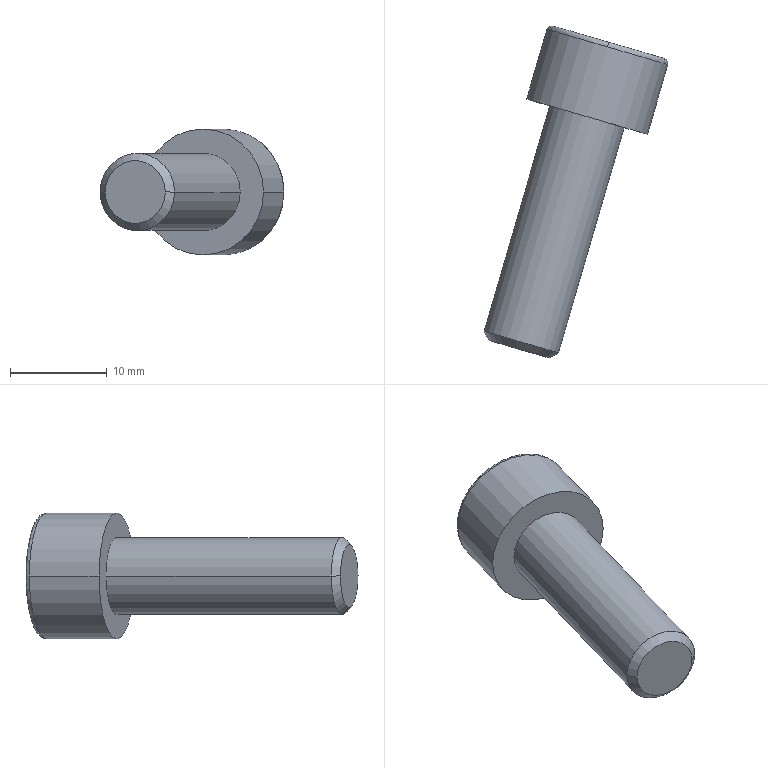Part | SolidWorks | features BaseBody 1 | 1 solid | 18 faces | box 18.984 x 34.285 x 13 mm | volume 2185 mm3 | plane 10 | cylinder 4 | cone 2 | spline 2 | commonest cylinder face diameters 8 x2 13 x2
STEP:
#1=CARTESIAN_POINT('',(22.625,457.214,-1.629));
#2=VERTEX_POINT('',#1);
#3=CARTESIAN_POINT('',(14.945,459.453,-1.629));
#4=VERTEX_POINT('',#3);
#5=CARTESIAN_POINT('',(18.785,458.333,-1.629));
#6=DIRECTION('',(-0.28,-0.96,0.));
#7=DIRECTION('',(0.96,-0.28,0.));
#8=AXIS2_PLACEMENT_3D('',#5,#6,#7);
#9=CIRCLE('',#8,4.);
#10=EDGE_CURVE('',#2,#4,#9,.T.);
#11=ORIENTED_EDGE('',*,*,#10,.T.);
#12=CARTESIAN_POINT('',(8.16,436.189,-1.629));
#13=VERTEX_POINT('',#12);
#14=CARTESIAN_POINT('',(11.553,447.821,-1.629));
#15=DIRECTION('',(-0.28,-0.96,0.));
#16=VECTOR('',#15,1000.);
#17=LINE('',#14,#16);
#18=EDGE_CURVE('',#4,#13,#17,.T.);
#19=ORIENTED_EDGE('',*,*,#18,.T.);
#20=CARTESIAN_POINT('',(15.841,433.95,-1.629));
#21=VERTEX_POINT('',#20);
#22=CARTESIAN_POINT('',(12.001,435.069,-1.629));
#23=DIRECTION('',(0.28,0.96,0.));
#24=DIRECTION('',(0.96,-0.28,0.));
#25=AXIS2_PLACEMENT_3D('',#22,#23,#24);
#26=CIRCLE('',#25,4.);
#27=EDGE_CURVE('',#13,#21,#26,.T.);
#28=ORIENTED_EDGE('',*,*,#27,.T.);
#29=CARTESIAN_POINT('',(19.233,445.582,-1.629));
#30=DIRECTION('',(-0.28,-0.96,0.));
#31=VECTOR('',#30,1000.);
#32=LINE('',#29,#31);
#33=EDGE_CURVE('',#2,#21,#32,.T.);
#34=ORIENTED_EDGE('',*,*,#33,.F.);
#35=EDGE_LOOP('',(#11,#19,#28,#34));
#36=FACE_OUTER_BOUND('',#35,.T.);
#37=CARTESIAN_POINT('',(15.393,446.701,-1.629));
#38=DIRECTION('',(-0.28,-0.96,0.));
#39=DIRECTION('',(0.96,-0.28,0.));
#40=AXIS2_PLACEMENT_3D('',#37,#38,#39);
#41=CYLINDRICAL_SURFACE('',#40,4.);
#42=ADVANCED_FACE('',(#36),#41,.T.);
#43=CARTESIAN_POINT('',(8.682,435.238,-1.629));
#44=VERTEX_POINT('',#43);
#45=CARTESIAN_POINT('',(14.89,433.428,-1.629));
#46=VERTEX_POINT('',#45);
#47=CARTESIAN_POINT('',(11.786,434.333,-1.629));
#48=DIRECTION('',(0.28,0.96,0.));
#49=DIRECTION('',(-0.96,0.28,0.));
#50=AXIS2_PLACEMENT_3D('',#47,#48,#49);
#51=CIRCLE('',#50,3.233);
#52=EDGE_CURVE('',#44,#46,#51,.T.);
#53=ORIENTED_EDGE('',*,*,#52,.T.);
#54=CARTESIAN_POINT('',(15.841,433.95,-1.629));
#55=DIRECTION('',(0.8768,0.4809,0.));
#56=VECTOR('',#55,1000.);
#57=LINE('',#54,#56);
#58=EDGE_CURVE('',#46,#21,#57,.T.);
#59=ORIENTED_EDGE('',*,*,#58,.T.);
#60=ORIENTED_EDGE('',*,*,#27,.F.);
#61=CARTESIAN_POINT('',(8.16,436.189,-1.629));
#62=DIRECTION('',(-0.4809,0.8768,0.));
#63=VECTOR('',#62,1000.);
#64=LINE('',#61,#63);
#65=EDGE_CURVE('',#44,#13,#64,.T.);
#66=ORIENTED_EDGE('',*,*,#65,.F.);
#67=EDGE_LOOP('',(#53,#59,#60,#66));
#68=FACE_OUTER_BOUND('',#67,.T.);
#69=CARTESIAN_POINT('',(12.001,435.069,-1.629));
#70=DIRECTION('',(0.28,0.96,0.));
#71=DIRECTION('',(-0.96,0.28,0.));
#72=AXIS2_PLACEMENT_3D('',#69,#70,#71);
#73=CONICAL_SURFACE('',#72,4.,0.7854);
#74=ADVANCED_FACE('',(#68),#73,.T.);
#75=CARTESIAN_POINT('',(20.884,465.534,4.871));
#76=VERTEX_POINT('',#75);
#77=CARTESIAN_POINT('',(14.644,467.353,-1.629));
#78=VERTEX_POINT('',#77);
#79=CARTESIAN_POINT('',(20.884,465.534,-1.629));
#80=DIRECTION('',(-0.28,-0.96,0.));
#81=DIRECTION('',(0.96,-0.28,0.));
#82=AXIS2_PLACEMENT_3D('',#79,#80,#81);
#83=CIRCLE('',#82,6.5);
#84=EDGE_CURVE('',#76,#78,#83,.T.);
#85=ORIENTED_EDGE('',*,*,#84,.T.);
#86=CARTESIAN_POINT('',(12.545,460.153,-1.629));
#87=VERTEX_POINT('',#86);
#88=CARTESIAN_POINT('',(13.594,463.753,-1.629));
#89=DIRECTION('',(-0.28,-0.96,0.));
#90=VECTOR('',#89,1000.);
#91=LINE('',#88,#90);
#92=EDGE_CURVE('',#78,#87,#91,.T.);
#93=ORIENTED_EDGE('',*,*,#92,.T.);
#94=CARTESIAN_POINT('',(25.025,456.514,-1.629));
#95=VERTEX_POINT('',#94);
#96=CARTESIAN_POINT('',(18.785,458.333,-1.629));
#97=DIRECTION('',(-0.28,-0.96,0.));
#98=DIRECTION('',(0.96,-0.28,0.));
#99=AXIS2_PLACEMENT_3D('',#96,#97,#98);
#100=CIRCLE('',#99,6.5);
#101=EDGE_CURVE('',#95,#87,#100,.T.);
#102=ORIENTED_EDGE('',*,*,#101,.F.);
#103=CARTESIAN_POINT('',(27.124,463.714,-1.629));
#104=VERTEX_POINT('',#103);
#105=CARTESIAN_POINT('',(26.075,460.114,-1.629));
#106=DIRECTION('',(-0.28,-0.96,0.));
#107=VECTOR('',#106,1000.);
#108=LINE('',#105,#107);
#109=EDGE_CURVE('',#104,#95,#108,.T.);
#110=ORIENTED_EDGE('',*,*,#109,.F.);
#111=CARTESIAN_POINT('',(20.884,465.534,-1.629));
#112=DIRECTION('',(-0.28,-0.96,0.));
#113=DIRECTION('',(0.96,-0.28,0.));
#114=AXIS2_PLACEMENT_3D('',#111,#112,#113);
#115=CIRCLE('',#114,6.5);
#116=EDGE_CURVE('',#104,#76,#115,.T.);
#117=ORIENTED_EDGE('',*,*,#116,.T.);
#118=EDGE_LOOP('',(#85,#93,#102,#110,#117));
#119=FACE_OUTER_BOUND('',#118,.T.);
#120=CARTESIAN_POINT('',(19.834,461.933,-1.629));
#121=DIRECTION('',(-0.28,-0.96,0.));
#122=DIRECTION('',(0.96,-0.28,0.));
#123=AXIS2_PLACEMENT_3D('',#120,#121,#122);
#124=CYLINDRICAL_SURFACE('',#123,6.5);
#125=ADVANCED_FACE('',(#119),#124,.T.);
#126=ORIENTED_EDGE('',*,*,#18,.F.);
#127=CARTESIAN_POINT('',(18.785,458.333,-1.629));
#128=DIRECTION('',(-0.28,-0.96,0.));
#129=DIRECTION('',(0.96,-0.28,0.));
#130=AXIS2_PLACEMENT_3D('',#127,#128,#129);
#131=CIRCLE('',#130,4.);
#132=EDGE_CURVE('',#4,#2,#131,.T.);
#133=ORIENTED_EDGE('',*,*,#132,.T.);
#134=ORIENTED_EDGE('',*,*,#33,.T.);
#135=CARTESIAN_POINT('',(12.001,435.069,-1.629));
#136=DIRECTION('',(0.28,0.96,0.));
#137=DIRECTION('',(0.96,-0.28,0.));
#138=AXIS2_PLACEMENT_3D('',#135,#136,#137);
#139=CIRCLE('',#138,4.);
#140=EDGE_CURVE('',#21,#13,#139,.T.);
#141=ORIENTED_EDGE('',*,*,#140,.T.);
#142=EDGE_LOOP('',(#126,#133,#134,#141));
#143=FACE_OUTER_BOUND('',#142,.T.);
#144=CARTESIAN_POINT('',(15.393,446.701,-1.629));
#145=DIRECTION('',(-0.28,-0.96,0.));
#146=DIRECTION('',(0.96,-0.28,0.));
#147=AXIS2_PLACEMENT_3D('',#144,#145,#146);
#148=CYLINDRICAL_SURFACE('',#147,4.);
#149=ADVANCED_FACE('',(#143),#148,.T.);
#150=ORIENTED_EDGE('',*,*,#58,.F.);
#151=CARTESIAN_POINT('',(11.786,434.333,-1.629));
#152=DIRECTION('',(0.28,0.96,0.));
#153=DIRECTION('',(-0.96,0.28,0.));
#154=AXIS2_PLACEMENT_3D('',#151,#152,#153);
#155=CIRCLE('',#154,3.233);
#156=EDGE_CURVE('',#46,#44,#155,.T.);
#157=ORIENTED_EDGE('',*,*,#156,.T.);
#158=ORIENTED_EDGE('',*,*,#65,.T.);
#159=ORIENTED_EDGE('',*,*,#140,.F.);
#160=EDGE_LOOP('',(#150,#157,#158,#159));
#161=FACE_OUTER_BOUND('',#160,.T.);
#162=CARTESIAN_POINT('',(12.001,435.069,-1.629));
#163=DIRECTION('',(0.28,0.96,0.));
#164=DIRECTION('',(-0.96,0.28,0.));
#165=AXIS2_PLACEMENT_3D('',#162,#163,#164);
#166=CONICAL_SURFACE('',#165,4.,0.7854);
#167=ADVANCED_FACE('',(#161),#166,.T.);
#168=ORIENTED_EDGE('',*,*,#101,.T.);
#169=CARTESIAN_POINT('',(18.785,458.333,-1.629));
#170=DIRECTION('',(-0.28,-0.96,0.));
#171=DIRECTION('',(0.96,-0.28,0.));
#172=AXIS2_PLACEMENT_3D('',#169,#170,#171);
#173=CIRCLE('',#172,6.5);
#174=EDGE_CURVE('',#87,#95,#173,.T.);
#175=ORIENTED_EDGE('',*,*,#174,.T.);
#176=EDGE_LOOP('',(#168,#175));
#177=FACE_OUTER_BOUND('',#176,.T.);
#178=ORIENTED_EDGE('',*,*,#10,.F.);
#179=ORIENTED_EDGE('',*,*,#132,.F.);
#180=EDGE_LOOP('',(#178,#179));
#181=FACE_BOUND('',#180,.T.);
#182=CARTESIAN_POINT('',(23.825,456.864,-1.629));
#183=DIRECTION('',(-0.28,-0.96,0.));
#184=DIRECTION('',(0.96,-0.28,0.));
#185=AXIS2_PLACEMENT_3D('',#182,#183,#184);
#186=PLANE('',#185);
#187=ADVANCED_FACE('',(#177,#181),#186,.T.);
#188=ORIENTED_EDGE('',*,*,#52,.F.);
#189=ORIENTED_EDGE('',*,*,#156,.F.);
#190=EDGE_LOOP('',(#188,#189));
#191=FACE_OUTER_BOUND('',#190,.T.);
#192=CARTESIAN_POINT('',(13.338,433.881,-1.629));
#193=DIRECTION('',(-0.28,-0.96,0.));
#194=DIRECTION('',(0.96,-0.28,0.));
#195=AXIS2_PLACEMENT_3D('',#192,#193,#194);
#196=PLANE('',#195);
#197=ADVANCED_FACE('',(#191),#196,.T.);
#198=ORIENTED_EDGE('',*,*,#92,.F.);
#199=CARTESIAN_POINT('',(20.884,465.534,-8.129));
#200=VERTEX_POINT('',#199);
#201=CARTESIAN_POINT('',(20.884,465.534,-1.629));
#202=DIRECTION('',(-0.28,-0.96,0.));
#203=DIRECTION('',(0.96,-0.28,0.));
#204=AXIS2_PLACEMENT_3D('',#201,#202,#203);
#205=CIRCLE('',#204,6.5);
#206=EDGE_CURVE('',#78,#200,#205,.T.);
#207=ORIENTED_EDGE('',*,*,#206,.T.);
#208=CARTESIAN_POINT('',(20.884,465.534,-1.629));
#209=DIRECTION('',(-0.28,-0.96,0.));
#210=DIRECTION('',(0.96,-0.28,0.));
#211=AXIS2_PLACEMENT_3D('',#208,#209,#210);
#212=CIRCLE('',#211,6.5);
#213=EDGE_CURVE('',#200,#104,#212,.T.);
#214=ORIENTED_EDGE('',*,*,#213,.T.);
#215=ORIENTED_EDGE('',*,*,#109,.T.);
#216=ORIENTED_EDGE('',*,*,#174,.F.);
#217=EDGE_LOOP('',(#198,#207,#214,#215,#216));
#218=FACE_OUTER_BOUND('',#217,.T.);
#219=CARTESIAN_POINT('',(19.834,461.933,-1.629));
#220=DIRECTION('',(-0.28,-0.96,0.));
#221=DIRECTION('',(0.96,-0.28,0.));
#222=AXIS2_PLACEMENT_3D('',#219,#220,#221);
#223=CYLINDRICAL_SURFACE('',#222,6.5);
#224=ADVANCED_FACE('',(#218),#223,.T.);
#225=ORIENTED_EDGE('',*,*,#84,.F.);
#226=CARTESIAN_POINT('',(21.024,466.014,4.371));
#227=VERTEX_POINT('',#226);
#228=CARTESIAN_POINT('',(20.884,465.534,4.871));
#229=CARTESIAN_POINT('',(20.966,465.815,4.871));
#230=CARTESIAN_POINT('',(21.024,466.014,4.664));
#231=CARTESIAN_POINT('',(21.024,466.014,4.371));
#232=(BOUNDED_CURVE()B_SPLINE_CURVE(3,(#228,#229,#230,#231),.UNSPECIFIED.,.F.,.F.)B_SPLINE_CURVE_WITH_KNOTS((4,4),(0.,1.455),.UNSPECIFIED.)CURVE()GEOMETRIC_REPRESENTATION_ITEM()RATIONAL_B_SPLINE_CURVE((1.,0.8047,0.8047,1.))REPRESENTATION_ITEM(''));
#233=EDGE_CURVE('',#76,#227,#232,.T.);
#234=ORIENTED_EDGE('',*,*,#233,.T.);
#235=CARTESIAN_POINT('',(21.024,466.014,-7.629));
#236=VERTEX_POINT('',#235);
#237=CARTESIAN_POINT('',(21.024,466.014,4.371));
#238=CARTESIAN_POINT('',(9.504,469.373,4.371));
#239=CARTESIAN_POINT('',(9.504,469.373,-7.629));
#240=CARTESIAN_POINT('',(21.024,466.014,-7.629));
#241=(BOUNDED_CURVE()B_SPLINE_CURVE(3,(#237,#238,#239,#240),.UNSPECIFIED.,.F.,.F.)B_SPLINE_CURVE_WITH_KNOTS((4,4),(0.,1.),.UNSPECIFIED.)CURVE()GEOMETRIC_REPRESENTATION_ITEM()RATIONAL_B_SPLINE_CURVE((1.,0.3333,0.3333,1.))REPRESENTATION_ITEM(''));
#242=EDGE_CURVE('',#227,#236,#241,.T.);
#243=ORIENTED_EDGE('',*,*,#242,.T.);
#244=CARTESIAN_POINT('',(21.024,466.014,-7.629));
#245=CARTESIAN_POINT('',(21.024,466.014,-7.922));
#246=CARTESIAN_POINT('',(20.966,465.815,-8.129));
#247=CARTESIAN_POINT('',(20.884,465.534,-8.129));
#248=(BOUNDED_CURVE()B_SPLINE_CURVE(3,(#244,#245,#246,#247),.UNSPECIFIED.,.F.,.F.)B_SPLINE_CURVE_WITH_KNOTS((4,4),(0.,1.455),.UNSPECIFIED.)CURVE()GEOMETRIC_REPRESENTATION_ITEM()RATIONAL_B_SPLINE_CURVE((1.,0.8047,0.8047,1.))REPRESENTATION_ITEM(''));
#249=EDGE_CURVE('',#236,#200,#248,.T.);
#250=ORIENTED_EDGE('',*,*,#249,.T.);
#251=ORIENTED_EDGE('',*,*,#206,.F.);
#252=EDGE_LOOP('',(#225,#234,#243,#250,#251));
#253=FACE_OUTER_BOUND('',#252,.T.);
#254=CARTESIAN_POINT('',(21.024,466.014,-7.629));
#255=CARTESIAN_POINT('',(9.504,469.373,-7.629));
#256=CARTESIAN_POINT('',(9.504,469.373,4.371));
#257=CARTESIAN_POINT('',(21.024,466.014,4.371));
#258=CARTESIAN_POINT('',(21.024,466.014,-7.922));
#259=CARTESIAN_POINT('',(8.942,469.537,-7.922));
#260=CARTESIAN_POINT('',(8.942,469.537,4.664));
#261=CARTESIAN_POINT('',(21.024,466.014,4.664));
#262=CARTESIAN_POINT('',(20.966,465.815,-8.129));
#263=CARTESIAN_POINT('',(8.486,469.454,-8.129));
#264=CARTESIAN_POINT('',(8.486,469.454,4.871));
#265=CARTESIAN_POINT('',(20.966,465.815,4.871));
#266=CARTESIAN_POINT('',(20.884,465.534,-8.129));
#267=CARTESIAN_POINT('',(8.404,469.173,-8.129));
#268=CARTESIAN_POINT('',(8.404,469.173,4.871));
#269=CARTESIAN_POINT('',(20.884,465.534,4.871));
#270=(BOUNDED_SURFACE()B_SPLINE_SURFACE(3,3,((#254,#255,#256,#257),(#258,#259,#260,#261),(#262,#263,#264,#265),(#266,#267,#268,#269)),.UNSPECIFIED.,.F.,.F.,.T.)B_SPLINE_SURFACE_WITH_KNOTS((4,4),(4,4),(0.,1.455),(0.,39.),.UNSPECIFIED.)GEOMETRIC_REPRESENTATION_ITEM()RATIONAL_B_SPLINE_SURFACE(((1.,0.3333,0.3333,1.),(0.8047,0.2682,0.2682,0.8047),(0.8047,0.2682,0.2682,0.8047),(1.,0.3333,0.3333,1.)))REPRESENTATION_ITEM('')SURFACE());
#271=ADVANCED_FACE('',(#253),#270,.T.);
#272=ORIENTED_EDGE('',*,*,#213,.F.);
#273=ORIENTED_EDGE('',*,*,#249,.F.);
#274=CARTESIAN_POINT('',(26.784,464.334,-1.629));
#275=VERTEX_POINT('',#274);
#276=CARTESIAN_POINT('',(21.024,466.014,-7.629));
#277=CARTESIAN_POINT('',(23.904,465.174,-7.629));
#278=CARTESIAN_POINT('',(26.784,464.334,-5.629));
#279=CARTESIAN_POINT('',(26.784,464.334,-1.629));
#280=(BOUNDED_CURVE()B_SPLINE_CURVE(3,(#276,#277,#278,#279),.UNSPECIFIED.,.F.,.F.)B_SPLINE_CURVE_WITH_KNOTS((4,4),(0.,1.),.UNSPECIFIED.)CURVE()GEOMETRIC_REPRESENTATION_ITEM()RATIONAL_B_SPLINE_CURVE((1.,0.6667,0.5,0.5))REPRESENTATION_ITEM(''));
#281=EDGE_CURVE('',#236,#275,#280,.T.);
#282=ORIENTED_EDGE('',*,*,#281,.T.);
#283=CARTESIAN_POINT('',(26.784,464.334,-1.629));
#284=CARTESIAN_POINT('',(26.784,464.334,2.371));
#285=CARTESIAN_POINT('',(23.904,465.174,4.371));
#286=CARTESIAN_POINT('',(21.024,466.014,4.371));
#287=(BOUNDED_CURVE()B_SPLINE_CURVE(3,(#283,#284,#285,#286),.UNSPECIFIED.,.F.,.F.)B_SPLINE_CURVE_WITH_KNOTS((4,4),(0.,1.),.UNSPECIFIED.)CURVE()GEOMETRIC_REPRESENTATION_ITEM()RATIONAL_B_SPLINE_CURVE((0.5,0.5,0.6667,1.))REPRESENTATION_ITEM(''));
#288=EDGE_CURVE('',#275,#227,#287,.T.);
#289=ORIENTED_EDGE('',*,*,#288,.T.);
#290=ORIENTED_EDGE('',*,*,#233,.F.);
#291=ORIENTED_EDGE('',*,*,#116,.F.);
#292=EDGE_LOOP('',(#272,#273,#282,#289,#290,#291));
#293=FACE_OUTER_BOUND('',#292,.T.);
#294=CARTESIAN_POINT('',(21.024,466.014,4.371));
#295=CARTESIAN_POINT('',(32.544,462.654,4.371));
#296=CARTESIAN_POINT('',(32.544,462.654,-7.629));
#297=CARTESIAN_POINT('',(21.024,466.014,-7.629));
#298=CARTESIAN_POINT('',(21.024,466.014,4.664));
#299=CARTESIAN_POINT('',(33.107,462.49,4.664));
#300=CARTESIAN_POINT('',(33.107,462.49,-7.922));
#301=CARTESIAN_POINT('',(21.024,466.014,-7.922));
#302=CARTESIAN_POINT('',(20.966,465.815,4.871));
#303=CARTESIAN_POINT('',(33.446,462.175,4.871));
#304=CARTESIAN_POINT('',(33.446,462.175,-8.129));
#305=CARTESIAN_POINT('',(20.966,465.815,-8.129));
#306=CARTESIAN_POINT('',(20.884,465.534,4.871));
#307=CARTESIAN_POINT('',(33.364,461.894,4.871));
#308=CARTESIAN_POINT('',(33.364,461.894,-8.129));
#309=CARTESIAN_POINT('',(20.884,465.534,-8.129));
#310=(BOUNDED_SURFACE()B_SPLINE_SURFACE(3,3,((#294,#295,#296,#297),(#298,#299,#300,#301),(#302,#303,#304,#305),(#306,#307,#308,#309)),.UNSPECIFIED.,.F.,.F.,.T.)B_SPLINE_SURFACE_WITH_KNOTS((4,4),(4,4),(0.,1.455),(0.,39.),.UNSPECIFIED.)GEOMETRIC_REPRESENTATION_ITEM()RATIONAL_B_SPLINE_SURFACE(((1.,0.3333,0.3333,1.),(0.8047,0.2682,0.2682,0.8047),(0.8047,0.2682,0.2682,0.8047),(1.,0.3333,0.3333,1.)))REPRESENTATION_ITEM('')SURFACE());
#311=ADVANCED_FACE('',(#293),#310,.T.);
#312=CARTESIAN_POINT('',(19.361,466.498,1.371));
#313=VERTEX_POINT('',#312);
#314=CARTESIAN_POINT('',(17.699,466.983,-1.629));
#315=VERTEX_POINT('',#314);
#316=CARTESIAN_POINT('',(19.361,466.498,1.371));
#317=DIRECTION('',(-0.48,0.14,-0.866));
#318=VECTOR('',#317,1000.);
#319=LINE('',#316,#318);
#320=EDGE_CURVE('',#313,#315,#319,.T.);
#321=ORIENTED_EDGE('',*,*,#320,.T.);
#322=CARTESIAN_POINT('',(19.361,466.498,-4.629));
#323=VERTEX_POINT('',#322);
#324=CARTESIAN_POINT('',(17.699,466.983,-1.629));
#325=DIRECTION('',(0.48,-0.14,-0.866));
#326=VECTOR('',#325,1000.);
#327=LINE('',#324,#326);
#328=EDGE_CURVE('',#315,#323,#327,.T.);
#329=ORIENTED_EDGE('',*,*,#328,.T.);
#330=CARTESIAN_POINT('',(22.687,465.529,-4.629));
#331=VERTEX_POINT('',#330);
#332=CARTESIAN_POINT('',(23.904,465.174,-4.629));
#333=DIRECTION('',(0.96,-0.28,0.));
#334=VECTOR('',#333,1000.);
#335=LINE('',#332,#334);
#336=EDGE_CURVE('',#323,#331,#335,.T.);
#337=ORIENTED_EDGE('',*,*,#336,.T.);
#338=CARTESIAN_POINT('',(24.35,465.044,-1.629));
#339=VERTEX_POINT('',#338);
#340=CARTESIAN_POINT('',(22.687,465.529,-4.629));
#341=DIRECTION('',(0.48,-0.14,0.866));
#342=VECTOR('',#341,1000.);
#343=LINE('',#340,#342);
#344=EDGE_CURVE('',#331,#339,#343,.T.);
#345=ORIENTED_EDGE('',*,*,#344,.T.);
#346=CARTESIAN_POINT('',(22.687,465.529,1.371));
#347=VERTEX_POINT('',#346);
#348=CARTESIAN_POINT('',(24.35,465.044,-1.629));
#349=DIRECTION('',(-0.48,0.14,0.866));
#350=VECTOR('',#349,1000.);
#351=LINE('',#348,#350);
#352=EDGE_CURVE('',#339,#347,#351,.T.);
#353=ORIENTED_EDGE('',*,*,#352,.T.);
#354=CARTESIAN_POINT('',(23.904,465.174,1.371));
#355=DIRECTION('',(-0.96,0.28,0.));
#356=VECTOR('',#355,1000.);
#357=LINE('',#354,#356);
#358=EDGE_CURVE('',#347,#313,#357,.T.);
#359=ORIENTED_EDGE('',*,*,#358,.T.);
#360=EDGE_LOOP('',(#321,#329,#337,#345,#353,#359));
#361=FACE_BOUND('',#360,.T.);
#362=ORIENTED_EDGE('',*,*,#288,.F.);
#363=ORIENTED_EDGE('',*,*,#281,.F.);
#364=ORIENTED_EDGE('',*,*,#242,.F.);
#365=EDGE_LOOP('',(#362,#363,#364));
#366=FACE_OUTER_BOUND('',#365,.T.);
#367=CARTESIAN_POINT('',(23.904,465.174,-1.629));
#368=DIRECTION('',(0.28,0.96,0.));
#369=DIRECTION('',(-0.96,0.28,0.));
#370=AXIS2_PLACEMENT_3D('',#367,#368,#369);
#371=PLANE('',#370);
#372=ADVANCED_FACE('',(#361,#366),#371,.T.);
#373=ORIENTED_EDGE('',*,*,#328,.F.);
#374=CARTESIAN_POINT('',(16.579,463.143,-1.629));
#375=VERTEX_POINT('',#374);
#376=CARTESIAN_POINT('',(16.579,463.143,-1.629));
#377=DIRECTION('',(0.28,0.96,0.));
#378=VECTOR('',#377,1000.);
#379=LINE('',#376,#378);
#380=EDGE_CURVE('',#375,#315,#379,.T.);
#381=ORIENTED_EDGE('',*,*,#380,.F.);
#382=CARTESIAN_POINT('',(18.242,462.658,-4.629));
#383=VERTEX_POINT('',#382);
#384=CARTESIAN_POINT('',(18.242,462.658,-4.629));
#385=DIRECTION('',(-0.48,0.14,0.866));
#386=VECTOR('',#385,1000.);
#387=LINE('',#384,#386);
#388=EDGE_CURVE('',#383,#375,#387,.T.);
#389=ORIENTED_EDGE('',*,*,#388,.F.);
#390=CARTESIAN_POINT('',(19.361,466.498,-4.629));
#391=DIRECTION('',(-0.28,-0.96,0.));
#392=VECTOR('',#391,1000.);
#393=LINE('',#390,#392);
#394=EDGE_CURVE('',#323,#383,#393,.T.);
#395=ORIENTED_EDGE('',*,*,#394,.F.);
#396=EDGE_LOOP('',(#373,#381,#389,#395));
#397=FACE_OUTER_BOUND('',#396,.T.);
#398=CARTESIAN_POINT('',(19.361,466.498,-4.629));
#399=DIRECTION('',(-0.8314,0.2424,-0.5));
#400=DIRECTION('',(-0.5154,0.,0.857));
#401=AXIS2_PLACEMENT_3D('',#398,#399,#400);
#402=PLANE('',#401);
#403=ADVANCED_FACE('',(#397),#402,.F.);
#404=ORIENTED_EDGE('',*,*,#320,.F.);
#405=CARTESIAN_POINT('',(18.242,462.658,1.371));
#406=VERTEX_POINT('',#405);
#407=CARTESIAN_POINT('',(18.242,462.658,1.371));
#408=DIRECTION('',(0.28,0.96,0.));
#409=VECTOR('',#408,1000.);
#410=LINE('',#407,#409);
#411=EDGE_CURVE('',#406,#313,#410,.T.);
#412=ORIENTED_EDGE('',*,*,#411,.F.);
#413=CARTESIAN_POINT('',(16.579,463.143,-1.629));
#414=DIRECTION('',(0.48,-0.14,0.866));
#415=VECTOR('',#414,1000.);
#416=LINE('',#413,#415);
#417=EDGE_CURVE('',#375,#406,#416,.T.);
#418=ORIENTED_EDGE('',*,*,#417,.F.);
#419=ORIENTED_EDGE('',*,*,#380,.T.);
#420=EDGE_LOOP('',(#404,#412,#418,#419));
#421=FACE_OUTER_BOUND('',#420,.T.);
#422=CARTESIAN_POINT('',(17.699,466.983,-1.629));
#423=DIRECTION('',(-0.8314,0.2424,0.5));
#424=DIRECTION('',(0.5154,0.,0.857));
#425=AXIS2_PLACEMENT_3D('',#422,#423,#424);
#426=PLANE('',#425);
#427=ADVANCED_FACE('',(#421),#426,.F.);
#428=ORIENTED_EDGE('',*,*,#358,.F.);
#429=CARTESIAN_POINT('',(21.567,461.689,1.371));
#430=VERTEX_POINT('',#429);
#431=CARTESIAN_POINT('',(21.567,461.689,1.371));
#432=DIRECTION('',(0.28,0.96,0.));
#433=VECTOR('',#432,1000.);
#434=LINE('',#431,#433);
#435=EDGE_CURVE('',#430,#347,#434,.T.);
#436=ORIENTED_EDGE('',*,*,#435,.F.);
#437=CARTESIAN_POINT('',(18.242,462.658,1.371));
#438=DIRECTION('',(0.96,-0.28,0.));
#439=VECTOR('',#438,1000.);
#440=LINE('',#437,#439);
#441=EDGE_CURVE('',#406,#430,#440,.T.);
#442=ORIENTED_EDGE('',*,*,#441,.F.);
#443=ORIENTED_EDGE('',*,*,#411,.T.);
#444=EDGE_LOOP('',(#428,#436,#442,#443));
#445=FACE_OUTER_BOUND('',#444,.T.);
#446=CARTESIAN_POINT('',(19.361,466.498,1.371));
#447=DIRECTION('',(0.,0.,1.));
#448=DIRECTION('',(1.,0.,0.));
#449=AXIS2_PLACEMENT_3D('',#446,#447,#448);
#450=PLANE('',#449);
#451=ADVANCED_FACE('',(#445),#450,.F.);
#452=ORIENTED_EDGE('',*,*,#352,.F.);
#453=CARTESIAN_POINT('',(23.23,461.204,-1.629));
#454=VERTEX_POINT('',#453);
#455=CARTESIAN_POINT('',(23.23,461.204,-1.629));
#456=DIRECTION('',(0.28,0.96,0.));
#457=VECTOR('',#456,1000.);
#458=LINE('',#455,#457);
#459=EDGE_CURVE('',#454,#339,#458,.T.);
#460=ORIENTED_EDGE('',*,*,#459,.F.);
#461=CARTESIAN_POINT('',(21.567,461.689,1.371));
#462=DIRECTION('',(0.48,-0.14,-0.866));
#463=VECTOR('',#462,1000.);
#464=LINE('',#461,#463);
#465=EDGE_CURVE('',#430,#454,#464,.T.);
#466=ORIENTED_EDGE('',*,*,#465,.F.);
#467=ORIENTED_EDGE('',*,*,#435,.T.);
#468=EDGE_LOOP('',(#452,#460,#466,#467));
#469=FACE_OUTER_BOUND('',#468,.T.);
#470=CARTESIAN_POINT('',(22.687,465.529,1.371));
#471=DIRECTION('',(0.8314,-0.2424,0.5));
#472=DIRECTION('',(0.5154,0.,-0.857));
#473=AXIS2_PLACEMENT_3D('',#470,#471,#472);
#474=PLANE('',#473);
#475=ADVANCED_FACE('',(#469),#474,.F.);
#476=ORIENTED_EDGE('',*,*,#344,.F.);
#477=CARTESIAN_POINT('',(21.567,461.689,-4.629));
#478=VERTEX_POINT('',#477);
#479=CARTESIAN_POINT('',(21.567,461.689,-4.629));
#480=DIRECTION('',(0.28,0.96,0.));
#481=VECTOR('',#480,1000.);
#482=LINE('',#479,#481);
#483=EDGE_CURVE('',#478,#331,#482,.T.);
#484=ORIENTED_EDGE('',*,*,#483,.F.);
#485=CARTESIAN_POINT('',(23.23,461.204,-1.629));
#486=DIRECTION('',(-0.48,0.14,-0.866));
#487=VECTOR('',#486,1000.);
#488=LINE('',#485,#487);
#489=EDGE_CURVE('',#454,#478,#488,.T.);
#490=ORIENTED_EDGE('',*,*,#489,.F.);
#491=ORIENTED_EDGE('',*,*,#459,.T.);
#492=EDGE_LOOP('',(#476,#484,#490,#491));
#493=FACE_OUTER_BOUND('',#492,.T.);
#494=CARTESIAN_POINT('',(24.35,465.044,-1.629));
#495=DIRECTION('',(0.8314,-0.2424,-0.5));
#496=DIRECTION('',(-0.5154,0.,-0.857));
#497=AXIS2_PLACEMENT_3D('',#494,#495,#496);
#498=PLANE('',#497);
#499=ADVANCED_FACE('',(#493),#498,.F.);
#500=ORIENTED_EDGE('',*,*,#336,.F.);
#501=ORIENTED_EDGE('',*,*,#394,.T.);
#502=CARTESIAN_POINT('',(21.567,461.689,-4.629));
#503=DIRECTION('',(-0.96,0.28,0.));
#504=VECTOR('',#503,1000.);
#505=LINE('',#502,#504);
#506=EDGE_CURVE('',#478,#383,#505,.T.);
#507=ORIENTED_EDGE('',*,*,#506,.F.);
#508=ORIENTED_EDGE('',*,*,#483,.T.);
#509=EDGE_LOOP('',(#500,#501,#507,#508));
#510=FACE_OUTER_BOUND('',#509,.T.);
#511=CARTESIAN_POINT('',(22.687,465.529,-4.629));
#512=DIRECTION('',(0.,0.,-1.));
#513=DIRECTION('',(-1.,0.,0.));
#514=AXIS2_PLACEMENT_3D('',#511,#512,#513);
#515=PLANE('',#514);
#516=ADVANCED_FACE('',(#510),#515,.F.);
#517=ORIENTED_EDGE('',*,*,#506,.T.);
#518=ORIENTED_EDGE('',*,*,#388,.T.);
#519=ORIENTED_EDGE('',*,*,#417,.T.);
#520=ORIENTED_EDGE('',*,*,#441,.T.);
#521=ORIENTED_EDGE('',*,*,#465,.T.);
#522=ORIENTED_EDGE('',*,*,#489,.T.);
#523=EDGE_LOOP('',(#517,#518,#519,#520,#521,#522));
#524=FACE_OUTER_BOUND('',#523,.T.);
#525=CARTESIAN_POINT('',(19.904,462.173,-1.629));
#526=DIRECTION('',(-0.28,-0.96,0.));
#527=DIRECTION('',(0.96,-0.28,0.));
#528=AXIS2_PLACEMENT_3D('',#525,#526,#527);
#529=PLANE('',#528);
#530=ADVANCED_FACE('',(#524),#529,.F.);
#531=CLOSED_SHELL('',(#42,#74,#125,#149,#167,#187,#197,#224,#271,#311,#372,#403,#427,#451,#475,#499,#516,#530));
#532=MANIFOLD_SOLID_BREP('',#531);
#533=CARTESIAN_POINT('',(0.,0.,0.));
#534=DIRECTION('',(0.,0.,1.));
#535=DIRECTION('',(1.,0.,0.));
#536=AXIS2_PLACEMENT_3D('',#533,#534,#535);
#537=(LENGTH_UNIT()NAMED_UNIT(*)SI_UNIT(.MILLI.,.METRE.));
#538=UNCERTAINTY_MEASURE_WITH_UNIT(LENGTH_MEASURE(0.00001),#537,'','');
#539=(NAMED_UNIT(*)PLANE_ANGLE_UNIT()SI_UNIT($,.RADIAN.));
#540=(NAMED_UNIT(*)SI_UNIT($,.STERADIAN.)SOLID_ANGLE_UNIT());
#541=(GEOMETRIC_REPRESENTATION_CONTEXT(3)GLOBAL_UNCERTAINTY_ASSIGNED_CONTEXT((#538))GLOBAL_UNIT_ASSIGNED_CONTEXT((#537,#539,#540))REPRESENTATION_CONTEXT('',''));
#542=ADVANCED_BREP_SHAPE_REPRESENTATION('',(#532,#536),#541);